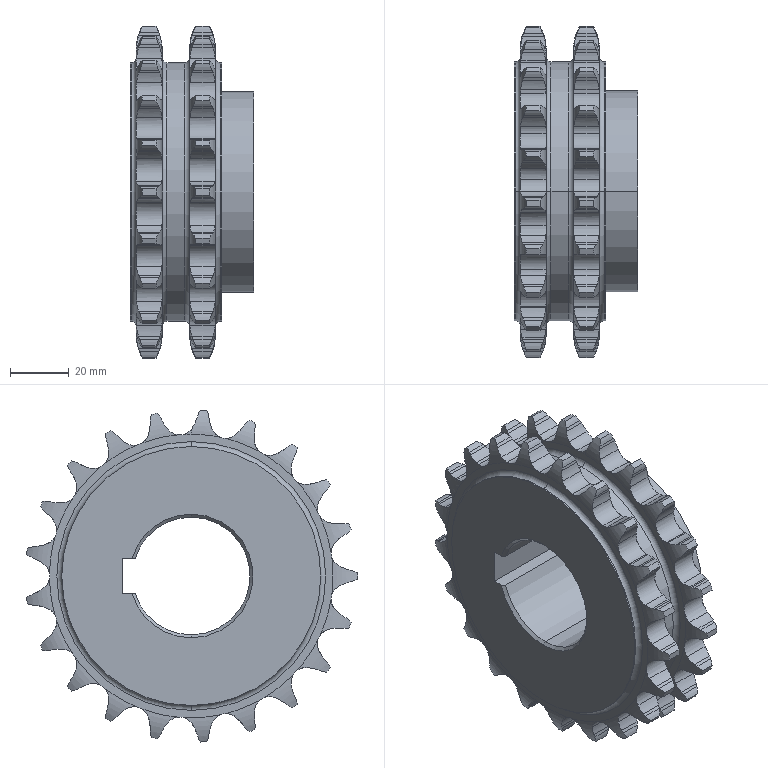Part | SolidWorks | features Revolution 3, Chamfer 2, Cut 2, CirPattern 1, LPattern 1 | 1 solid | 479 faces | box 42 x 112.513 x 112.819 mm | volume 211339 mm3 | cylinder 283 | torus 96 | plane 94 | cone 6 | commonest cylinder face diameters 14.747 x88 26.567 x88 10.311 x54 113 x42 88 x6 40 x3